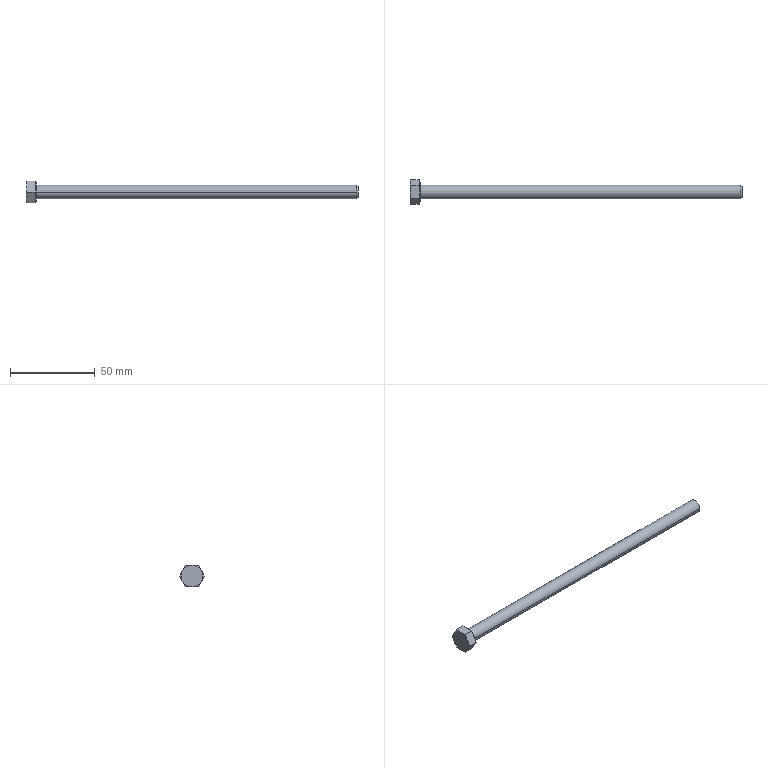Part | SolidWorks | features BaseBody 1 | 1 solid | 28 faces | box 195.95 x 14.699 x 12.73 mm | volume 10367 mm3 | plane 15 | cone 11 | cylinder 2 | commonest cylinder face diameters 8 x2
STEP:
#1=CARTESIAN_POINT('',(195.95,3.324,0.));
#2=VERTEX_POINT('',#1);
#3=CARTESIAN_POINT('',(195.95,-3.323,0.));
#4=VERTEX_POINT('',#3);
#5=CARTESIAN_POINT('',(195.95,0.,0.));
#6=DIRECTION('',(1.,0.,0.));
#7=DIRECTION('',(0.,1.,0.));
#8=AXIS2_PLACEMENT_3D('',#5,#6,#7);
#9=CIRCLE('',#8,3.324);
#10=EDGE_CURVE('',#2,#4,#9,.T.);
#11=ORIENTED_EDGE('',*,*,#10,.F.);
#12=CARTESIAN_POINT('',(195.273,4.,0.));
#13=VERTEX_POINT('',#12);
#14=CARTESIAN_POINT('',(195.95,3.324,0.));
#15=DIRECTION('',(-0.7071,0.7071,0.));
#16=VECTOR('',#15,1000.);
#17=LINE('',#14,#16);
#18=EDGE_CURVE('',#2,#13,#17,.T.);
#19=ORIENTED_EDGE('',*,*,#18,.T.);
#20=CARTESIAN_POINT('',(195.273,-4.,0.));
#21=VERTEX_POINT('',#20);
#22=CARTESIAN_POINT('',(195.273,0.,0.));
#23=DIRECTION('',(-1.,0.,0.));
#24=DIRECTION('',(0.,1.,0.));
#25=AXIS2_PLACEMENT_3D('',#22,#23,#24);
#26=CIRCLE('',#25,4.);
#27=EDGE_CURVE('',#21,#13,#26,.T.);
#28=ORIENTED_EDGE('',*,*,#27,.F.);
#29=CARTESIAN_POINT('',(195.95,-3.323,0.));
#30=DIRECTION('',(-0.7071,-0.7071,0.));
#31=VECTOR('',#30,1000.);
#32=LINE('',#29,#31);
#33=EDGE_CURVE('',#4,#21,#32,.T.);
#34=ORIENTED_EDGE('',*,*,#33,.F.);
#35=EDGE_LOOP('',(#11,#19,#28,#34));
#36=FACE_OUTER_BOUND('',#35,.T.);
#37=CARTESIAN_POINT('',(195.95,0.,0.));
#38=DIRECTION('',(-1.,0.,0.));
#39=DIRECTION('',(0.,-1.,0.));
#40=AXIS2_PLACEMENT_3D('',#37,#38,#39);
#41=CONICAL_SURFACE('',#40,3.324,0.7854);
#42=ADVANCED_FACE('',(#36),#41,.T.);
#43=ORIENTED_EDGE('',*,*,#27,.T.);
#44=CARTESIAN_POINT('',(5.95,4.,0.));
#45=VERTEX_POINT('',#44);
#46=CARTESIAN_POINT('',(195.95,4.,0.));
#47=DIRECTION('',(-1.,0.,0.));
#48=VECTOR('',#47,1000.);
#49=LINE('',#46,#48);
#50=EDGE_CURVE('',#13,#45,#49,.T.);
#51=ORIENTED_EDGE('',*,*,#50,.T.);
#52=CARTESIAN_POINT('',(5.95,-4.,0.));
#53=VERTEX_POINT('',#52);
#54=CARTESIAN_POINT('',(5.95,0.,0.));
#55=DIRECTION('',(1.,0.,0.));
#56=DIRECTION('',(0.,-1.,0.));
#57=AXIS2_PLACEMENT_3D('',#54,#55,#56);
#58=CIRCLE('',#57,4.);
#59=EDGE_CURVE('',#45,#53,#58,.T.);
#60=ORIENTED_EDGE('',*,*,#59,.T.);
#61=CARTESIAN_POINT('',(195.95,-4.,0.));
#62=DIRECTION('',(-1.,0.,0.));
#63=VECTOR('',#62,1000.);
#64=LINE('',#61,#63);
#65=EDGE_CURVE('',#21,#53,#64,.T.);
#66=ORIENTED_EDGE('',*,*,#65,.F.);
#67=EDGE_LOOP('',(#43,#51,#60,#66));
#68=FACE_OUTER_BOUND('',#67,.T.);
#69=CARTESIAN_POINT('',(195.95,0.,0.));
#70=DIRECTION('',(-1.,0.,0.));
#71=DIRECTION('',(0.,-1.,0.));
#72=AXIS2_PLACEMENT_3D('',#69,#70,#71);
#73=CYLINDRICAL_SURFACE('',#72,4.);
#74=ADVANCED_FACE('',(#68),#73,.T.);
#75=CARTESIAN_POINT('',(5.95,-5.815,0.));
#76=VERTEX_POINT('',#75);
#77=CARTESIAN_POINT('',(5.95,5.815,0.));
#78=VERTEX_POINT('',#77);
#79=CARTESIAN_POINT('',(5.95,0.,0.));
#80=DIRECTION('',(-1.,0.,0.));
#81=DIRECTION('',(0.,-1.,0.));
#82=AXIS2_PLACEMENT_3D('',#79,#80,#81);
#83=CIRCLE('',#82,5.815);
#84=EDGE_CURVE('',#76,#78,#83,.T.);
#85=ORIENTED_EDGE('',*,*,#84,.T.);
#86=CARTESIAN_POINT('',(5.45,6.365,0.));
#87=VERTEX_POINT('',#86);
#88=CARTESIAN_POINT('',(5.95,5.815,0.));
#89=DIRECTION('',(-0.6727,0.7399,0.));
#90=VECTOR('',#89,1000.);
#91=LINE('',#88,#90);
#92=EDGE_CURVE('',#78,#87,#91,.T.);
#93=ORIENTED_EDGE('',*,*,#92,.T.);
#94=CARTESIAN_POINT('',(5.45,5.512,3.183));
#95=VERTEX_POINT('',#94);
#96=CARTESIAN_POINT('',(5.45,0.,0.));
#97=DIRECTION('',(-1.,0.,0.));
#98=DIRECTION('',(0.,-1.,0.));
#99=AXIS2_PLACEMENT_3D('',#96,#97,#98);
#100=CIRCLE('',#99,6.365);
#101=EDGE_CURVE('',#95,#87,#100,.T.);
#102=ORIENTED_EDGE('',*,*,#101,.F.);
#103=CARTESIAN_POINT('',(5.45,0.,6.365));
#104=VERTEX_POINT('',#103);
#105=CARTESIAN_POINT('',(5.45,0.,0.));
#106=DIRECTION('',(-1.,0.,0.));
#107=DIRECTION('',(0.,-1.,0.));
#108=AXIS2_PLACEMENT_3D('',#105,#106,#107);
#109=CIRCLE('',#108,6.365);
#110=EDGE_CURVE('',#104,#95,#109,.T.);
#111=ORIENTED_EDGE('',*,*,#110,.F.);
#112=CARTESIAN_POINT('',(5.45,-5.512,3.183));
#113=VERTEX_POINT('',#112);
#114=CARTESIAN_POINT('',(5.45,0.,0.));
#115=DIRECTION('',(-1.,0.,0.));
#116=DIRECTION('',(0.,-1.,0.));
#117=AXIS2_PLACEMENT_3D('',#114,#115,#116);
#118=CIRCLE('',#117,6.365);
#119=EDGE_CURVE('',#113,#104,#118,.T.);
#120=ORIENTED_EDGE('',*,*,#119,.F.);
#121=CARTESIAN_POINT('',(5.45,-6.365,0.));
#122=VERTEX_POINT('',#121);
#123=CARTESIAN_POINT('',(5.45,0.,0.));
#124=DIRECTION('',(-1.,0.,0.));
#125=DIRECTION('',(0.,-1.,0.));
#126=AXIS2_PLACEMENT_3D('',#123,#124,#125);
#127=CIRCLE('',#126,6.365);
#128=EDGE_CURVE('',#122,#113,#127,.T.);
#129=ORIENTED_EDGE('',*,*,#128,.F.);
#130=CARTESIAN_POINT('',(5.95,-5.815,0.));
#131=DIRECTION('',(-0.6727,-0.7399,0.));
#132=VECTOR('',#131,1000.);
#133=LINE('',#130,#132);
#134=EDGE_CURVE('',#76,#122,#133,.T.);
#135=ORIENTED_EDGE('',*,*,#134,.F.);
#136=EDGE_LOOP('',(#85,#93,#102,#111,#120,#129,#135));
#137=FACE_OUTER_BOUND('',#136,.T.);
#138=CARTESIAN_POINT('',(5.95,0.,0.));
#139=DIRECTION('',(-1.,0.,0.));
#140=DIRECTION('',(0.,-1.,0.));
#141=AXIS2_PLACEMENT_3D('',#138,#139,#140);
#142=CONICAL_SURFACE('',#141,5.815,0.833);
#143=ADVANCED_FACE('',(#137),#142,.T.);
#144=CARTESIAN_POINT('',(0.,6.365,0.));
#145=VERTEX_POINT('',#144);
#146=CARTESIAN_POINT('',(0.,5.512,-3.183));
#147=VERTEX_POINT('',#146);
#148=CARTESIAN_POINT('',(0.,0.,0.));
#149=DIRECTION('',(-1.,0.,0.));
#150=DIRECTION('',(0.,0.,1.));
#151=AXIS2_PLACEMENT_3D('',#148,#149,#150);
#152=CIRCLE('',#151,6.365);
#153=EDGE_CURVE('',#145,#147,#152,.T.);
#154=ORIENTED_EDGE('',*,*,#153,.F.);
#155=CARTESIAN_POINT('',(0.3584,7.35,0.));
#156=VERTEX_POINT('',#155);
#157=CARTESIAN_POINT('',(0.,6.365,0.));
#158=DIRECTION('',(0.342,0.9397,0.));
#159=VECTOR('',#158,1000.);
#160=LINE('',#157,#159);
#161=EDGE_CURVE('',#145,#156,#160,.T.);
#162=ORIENTED_EDGE('',*,*,#161,.T.);
#163=CARTESIAN_POINT('',(0.3584,7.35,0.));
#164=CARTESIAN_POINT('',(0.3008,7.191,-0.2742));
#165=CARTESIAN_POINT('',(0.25,7.037,-0.5421));
#166=CARTESIAN_POINT('',(0.184,6.808,-0.9385));
#167=CARTESIAN_POINT('',(0.1638,6.732,-1.07));
#168=CARTESIAN_POINT('',(0.1359,6.619,-1.266));
#169=CARTESIAN_POINT('',(0.127,6.581,-1.331));
#170=CARTESIAN_POINT('',(0.1102,6.506,-1.461));
#171=CARTESIAN_POINT('',(0.1024,6.47,-1.524));
#172=CARTESIAN_POINT('',(0.07901,6.354,-1.725));
#173=CARTESIAN_POINT('',(0.06534,6.277,-1.858));
#174=CARTESIAN_POINT('',(0.04182,6.124,-2.123));
#175=CARTESIAN_POINT('',(0.03203,6.049,-2.254));
#176=CARTESIAN_POINT('',(0.008007,5.818,-2.654));
#177=CARTESIAN_POINT('',(0.,5.666,-2.917));
#178=CARTESIAN_POINT('',(0.,5.512,-3.183));
#179=B_SPLINE_CURVE_WITH_KNOTS('',3,(#163,#164,#165,#166,#167,#168,#169,#170,#171,#172,#173,#174,#175,#176,#177,#178),.UNSPECIFIED.,.F.,.F.,(4,2,2,2,2,2,2,4),(0.,0.25,0.375,0.4375,0.5,0.625,0.75,1.),.UNSPECIFIED.);
#180=EDGE_CURVE('',#156,#147,#179,.T.);
#181=ORIENTED_EDGE('',*,*,#180,.T.);
#182=EDGE_LOOP('',(#154,#162,#181));
#183=FACE_OUTER_BOUND('',#182,.T.);
#184=CARTESIAN_POINT('',(0.,0.,0.));
#185=DIRECTION('',(1.,0.,0.));
#186=DIRECTION('',(0.,1.,0.));
#187=AXIS2_PLACEMENT_3D('',#184,#185,#186);
#188=CONICAL_SURFACE('',#187,6.365,1.222);
#189=ADVANCED_FACE('',(#183),#188,.T.);
#190=ORIENTED_EDGE('',*,*,#84,.F.);
#191=CARTESIAN_POINT('',(5.95,0.,0.));
#192=DIRECTION('',(-1.,0.,0.));
#193=DIRECTION('',(0.,-1.,0.));
#194=AXIS2_PLACEMENT_3D('',#191,#192,#193);
#195=CIRCLE('',#194,5.815);
#196=EDGE_CURVE('',#78,#76,#195,.T.);
#197=ORIENTED_EDGE('',*,*,#196,.F.);
#198=EDGE_LOOP('',(#190,#197));
#199=FACE_OUTER_BOUND('',#198,.T.);
#200=CARTESIAN_POINT('',(5.95,0.,0.));
#201=DIRECTION('',(1.,0.,0.));
#202=DIRECTION('',(0.,-1.,0.));
#203=AXIS2_PLACEMENT_3D('',#200,#201,#202);
#204=CIRCLE('',#203,4.);
#205=EDGE_CURVE('',#53,#45,#204,.T.);
#206=ORIENTED_EDGE('',*,*,#205,.F.);
#207=ORIENTED_EDGE('',*,*,#59,.F.);
#208=EDGE_LOOP('',(#206,#207));
#209=FACE_BOUND('',#208,.T.);
#210=CARTESIAN_POINT('',(5.95,0.,0.));
#211=DIRECTION('',(-1.,0.,0.));
#212=DIRECTION('',(0.,1.,0.));
#213=AXIS2_PLACEMENT_3D('',#210,#211,#212);
#214=PLANE('',#213);
#215=ADVANCED_FACE('',(#199,#209),#214,.F.);
#216=CARTESIAN_POINT('',(5.45,-3.675,6.365));
#217=VERTEX_POINT('',#216);
#218=CARTESIAN_POINT('',(5.45,-3.675,6.365));
#219=DIRECTION('',(0.,-0.5,-0.866));
#220=VECTOR('',#219,1000.);
#221=LINE('',#218,#220);
#222=EDGE_CURVE('',#217,#113,#221,.T.);
#223=ORIENTED_EDGE('',*,*,#222,.T.);
#224=ORIENTED_EDGE('',*,*,#119,.T.);
#225=CARTESIAN_POINT('',(5.45,3.675,6.365));
#226=DIRECTION('',(0.,-1.,0.));
#227=VECTOR('',#226,1000.);
#228=LINE('',#225,#227);
#229=EDGE_CURVE('',#104,#217,#228,.T.);
#230=ORIENTED_EDGE('',*,*,#229,.T.);
#231=EDGE_LOOP('',(#223,#224,#230));
#232=FACE_OUTER_BOUND('',#231,.T.);
#233=CARTESIAN_POINT('',(5.45,0.,12.73));
#234=DIRECTION('',(-1.,0.,0.));
#235=DIRECTION('',(0.,0.,1.));
#236=AXIS2_PLACEMENT_3D('',#233,#234,#235);
#237=PLANE('',#236);
#238=ADVANCED_FACE('',(#232),#237,.F.);
#239=CARTESIAN_POINT('',(5.45,3.675,6.365));
#240=VERTEX_POINT('',#239);
#241=CARTESIAN_POINT('',(5.45,3.675,6.365));
#242=DIRECTION('',(0.,-1.,0.));
#243=VECTOR('',#242,1000.);
#244=LINE('',#241,#243);
#245=EDGE_CURVE('',#240,#104,#244,.T.);
#246=ORIENTED_EDGE('',*,*,#245,.T.);
#247=ORIENTED_EDGE('',*,*,#110,.T.);
#248=CARTESIAN_POINT('',(5.45,7.35,0.));
#249=DIRECTION('',(0.,-0.5,0.866));
#250=VECTOR('',#249,1000.);
#251=LINE('',#248,#250);
#252=EDGE_CURVE('',#95,#240,#251,.T.);
#253=ORIENTED_EDGE('',*,*,#252,.T.);
#254=EDGE_LOOP('',(#246,#247,#253));
#255=FACE_OUTER_BOUND('',#254,.T.);
#256=CARTESIAN_POINT('',(5.45,0.,12.73));
#257=DIRECTION('',(-1.,0.,0.));
#258=DIRECTION('',(0.,0.,1.));
#259=AXIS2_PLACEMENT_3D('',#256,#257,#258);
#260=PLANE('',#259);
#261=ADVANCED_FACE('',(#255),#260,.F.);
#262=CARTESIAN_POINT('',(5.45,7.35,0.));
#263=VERTEX_POINT('',#262);
#264=CARTESIAN_POINT('',(5.45,7.35,0.));
#265=DIRECTION('',(0.,-0.5,0.866));
#266=VECTOR('',#265,1000.);
#267=LINE('',#264,#266);
#268=EDGE_CURVE('',#263,#95,#267,.T.);
#269=ORIENTED_EDGE('',*,*,#268,.T.);
#270=ORIENTED_EDGE('',*,*,#101,.T.);
#271=CARTESIAN_POINT('',(5.45,5.512,-3.183));
#272=VERTEX_POINT('',#271);
#273=CARTESIAN_POINT('',(5.45,0.,0.));
#274=DIRECTION('',(-1.,0.,0.));
#275=DIRECTION('',(0.,-1.,0.));
#276=AXIS2_PLACEMENT_3D('',#273,#274,#275);
#277=CIRCLE('',#276,6.365);
#278=EDGE_CURVE('',#87,#272,#277,.T.);
#279=ORIENTED_EDGE('',*,*,#278,.T.);
#280=CARTESIAN_POINT('',(5.45,3.675,-6.365));
#281=DIRECTION('',(0.,0.5,0.866));
#282=VECTOR('',#281,1000.);
#283=LINE('',#280,#282);
#284=EDGE_CURVE('',#272,#263,#283,.T.);
#285=ORIENTED_EDGE('',*,*,#284,.T.);
#286=EDGE_LOOP('',(#269,#270,#279,#285));
#287=FACE_OUTER_BOUND('',#286,.T.);
#288=CARTESIAN_POINT('',(5.45,0.,12.73));
#289=DIRECTION('',(-1.,0.,0.));
#290=DIRECTION('',(0.,0.,1.));
#291=AXIS2_PLACEMENT_3D('',#288,#289,#290);
#292=PLANE('',#291);
#293=ADVANCED_FACE('',(#287),#292,.F.);
#294=CARTESIAN_POINT('',(5.45,3.675,-6.365));
#295=VERTEX_POINT('',#294);
#296=CARTESIAN_POINT('',(5.45,3.675,-6.365));
#297=DIRECTION('',(0.,0.5,0.866));
#298=VECTOR('',#297,1000.);
#299=LINE('',#296,#298);
#300=EDGE_CURVE('',#295,#272,#299,.T.);
#301=ORIENTED_EDGE('',*,*,#300,.T.);
#302=CARTESIAN_POINT('',(5.45,0.,-6.365));
#303=VERTEX_POINT('',#302);
#304=CARTESIAN_POINT('',(5.45,0.,0.));
#305=DIRECTION('',(-1.,0.,0.));
#306=DIRECTION('',(0.,-1.,0.));
#307=AXIS2_PLACEMENT_3D('',#304,#305,#306);
#308=CIRCLE('',#307,6.365);
#309=EDGE_CURVE('',#272,#303,#308,.T.);
#310=ORIENTED_EDGE('',*,*,#309,.T.);
#311=CARTESIAN_POINT('',(5.45,-3.675,-6.365));
#312=DIRECTION('',(0.,1.,0.));
#313=VECTOR('',#312,1000.);
#314=LINE('',#311,#313);
#315=EDGE_CURVE('',#303,#295,#314,.T.);
#316=ORIENTED_EDGE('',*,*,#315,.T.);
#317=EDGE_LOOP('',(#301,#310,#316));
#318=FACE_OUTER_BOUND('',#317,.T.);
#319=CARTESIAN_POINT('',(5.45,0.,12.73));
#320=DIRECTION('',(-1.,0.,0.));
#321=DIRECTION('',(0.,0.,1.));
#322=AXIS2_PLACEMENT_3D('',#319,#320,#321);
#323=PLANE('',#322);
#324=ADVANCED_FACE('',(#318),#323,.F.);
#325=CARTESIAN_POINT('',(5.45,-3.675,-6.365));
#326=VERTEX_POINT('',#325);
#327=CARTESIAN_POINT('',(5.45,-3.675,-6.365));
#328=DIRECTION('',(0.,1.,0.));
#329=VECTOR('',#328,1000.);
#330=LINE('',#327,#329);
#331=EDGE_CURVE('',#326,#303,#330,.T.);
#332=ORIENTED_EDGE('',*,*,#331,.T.);
#333=CARTESIAN_POINT('',(5.45,-5.512,-3.183));
#334=VERTEX_POINT('',#333);
#335=CARTESIAN_POINT('',(5.45,0.,0.));
#336=DIRECTION('',(-1.,0.,0.));
#337=DIRECTION('',(0.,-1.,0.));
#338=AXIS2_PLACEMENT_3D('',#335,#336,#337);
#339=CIRCLE('',#338,6.365);
#340=EDGE_CURVE('',#303,#334,#339,.T.);
#341=ORIENTED_EDGE('',*,*,#340,.T.);
#342=CARTESIAN_POINT('',(5.45,-7.35,0.));
#343=DIRECTION('',(0.,0.5,-0.866));
#344=VECTOR('',#343,1000.);
#345=LINE('',#342,#344);
#346=EDGE_CURVE('',#334,#326,#345,.T.);
#347=ORIENTED_EDGE('',*,*,#346,.T.);
#348=EDGE_LOOP('',(#332,#341,#347));
#349=FACE_OUTER_BOUND('',#348,.T.);
#350=CARTESIAN_POINT('',(5.45,0.,12.73));
#351=DIRECTION('',(-1.,0.,0.));
#352=DIRECTION('',(0.,0.,1.));
#353=AXIS2_PLACEMENT_3D('',#350,#351,#352);
#354=PLANE('',#353);
#355=ADVANCED_FACE('',(#349),#354,.F.);
#356=CARTESIAN_POINT('',(0.3584,-7.35,0.));
#357=VERTEX_POINT('',#356);
#358=CARTESIAN_POINT('',(0.,-5.512,3.183));
#359=VERTEX_POINT('',#358);
#360=CARTESIAN_POINT('',(0.3584,-7.35,0.));
#361=CARTESIAN_POINT('',(0.3008,-7.191,0.2742));
#362=CARTESIAN_POINT('',(0.25,-7.037,0.5421));
#363=CARTESIAN_POINT('',(0.184,-6.808,0.9385));
#364=CARTESIAN_POINT('',(0.1638,-6.732,1.07));
#365=CARTESIAN_POINT('',(0.1359,-6.619,1.266));
#366=CARTESIAN_POINT('',(0.127,-6.581,1.331));
#367=CARTESIAN_POINT('',(0.1102,-6.506,1.461));
#368=CARTESIAN_POINT('',(0.1024,-6.47,1.524));
#369=CARTESIAN_POINT('',(0.07901,-6.354,1.725));
#370=CARTESIAN_POINT('',(0.06534,-6.277,1.858));
#371=CARTESIAN_POINT('',(0.04182,-6.124,2.123));
#372=CARTESIAN_POINT('',(0.03203,-6.049,2.254));
#373=CARTESIAN_POINT('',(0.008007,-5.818,2.654));
#374=CARTESIAN_POINT('',(0.,-5.666,2.917));
#375=CARTESIAN_POINT('',(0.,-5.512,3.183));
#376=B_SPLINE_CURVE_WITH_KNOTS('',3,(#360,#361,#362,#363,#364,#365,#366,#367,#368,#369,#370,#371,#372,#373,#374,#375),.UNSPECIFIED.,.F.,.F.,(4,2,2,2,2,2,2,4),(0.,0.25,0.375,0.4375,0.5,0.625,0.75,1.),.UNSPECIFIED.);
#377=EDGE_CURVE('',#357,#359,#376,.T.);
#378=ORIENTED_EDGE('',*,*,#377,.F.);
#379=CARTESIAN_POINT('',(5.45,-7.35,0.));
#380=VERTEX_POINT('',#379);
#381=CARTESIAN_POINT('',(5.45,-7.35,0.));
#382=DIRECTION('',(-1.,0.,0.));
#383=VECTOR('',#382,1000.);
#384=LINE('',#381,#383);
#385=EDGE_CURVE('',#380,#357,#384,.T.);
#386=ORIENTED_EDGE('',*,*,#385,.F.);
#387=CARTESIAN_POINT('',(5.45,-3.675,6.365));
#388=DIRECTION('',(0.,-0.5,-0.866));
#389=VECTOR('',#388,1000.);
#390=LINE('',#387,#389);
#391=EDGE_CURVE('',#113,#380,#390,.T.);
#392=ORIENTED_EDGE('',*,*,#391,.F.);
#393=ORIENTED_EDGE('',*,*,#222,.F.);
#394=CARTESIAN_POINT('',(0.3584,-3.675,6.365));
#395=VERTEX_POINT('',#394);
#396=CARTESIAN_POINT('',(5.45,-3.675,6.365));
#397=DIRECTION('',(-1.,0.,0.));
#398=VECTOR('',#397,1000.);
#399=LINE('',#396,#398);
#400=EDGE_CURVE('',#217,#395,#399,.T.);
#401=ORIENTED_EDGE('',*,*,#400,.T.);
#402=CARTESIAN_POINT('',(0.,-5.512,3.183));
#403=CARTESIAN_POINT('',(0.,-5.436,3.315));
#404=CARTESIAN_POINT('',(0.002002,-5.359,3.447));
#405=CARTESIAN_POINT('',(0.01001,-5.206,3.712));
#406=CARTESIAN_POINT('',(0.01608,-5.129,3.846));
#407=CARTESIAN_POINT('',(0.03196,-4.977,4.11));
#408=CARTESIAN_POINT('',(0.04181,-4.9,4.242));
#409=CARTESIAN_POINT('',(0.05946,-4.786,4.441));
#410=CARTESIAN_POINT('',(0.06582,-4.747,4.507));
#411=CARTESIAN_POINT('',(0.07949,-4.671,4.64));
#412=CARTESIAN_POINT('',(0.08702,-4.631,4.709));
#413=CARTESIAN_POINT('',(0.1552,-4.293,5.294));
#414=CARTESIAN_POINT('',(0.2431,-3.991,5.817));
#415=CARTESIAN_POINT('',(0.3584,-3.675,6.365));
#416=B_SPLINE_CURVE_WITH_KNOTS('',3,(#402,#403,#404,#405,#406,#407,#408,#409,#410,#411,#412,#413,#414,#415),.UNSPECIFIED.,.F.,.F.,(4,2,2,2,2,2,4),(0.,0.125,0.25,0.375,0.4375,0.5,1.),.UNSPECIFIED.);
#417=EDGE_CURVE('',#359,#395,#416,.T.);
#418=ORIENTED_EDGE('',*,*,#417,.F.);
#419=EDGE_LOOP('',(#378,#386,#392,#393,#401,#418));
#420=FACE_OUTER_BOUND('',#419,.T.);
#421=CARTESIAN_POINT('',(5.45,-3.675,6.365));
#422=DIRECTION('',(0.,0.866,-0.5));
#423=DIRECTION('',(-1.,0.,0.));
#424=AXIS2_PLACEMENT_3D('',#421,#422,#423);
#425=PLANE('',#424);
#426=ADVANCED_FACE('',(#420),#425,.F.);
#427=CARTESIAN_POINT('',(0.3584,-3.675,-6.365));
#428=VERTEX_POINT('',#427);
#429=CARTESIAN_POINT('',(0.,-5.512,-3.183));
#430=VERTEX_POINT('',#429);
#431=CARTESIAN_POINT('',(0.3584,-3.675,-6.365));
#432=CARTESIAN_POINT('',(0.3008,-3.833,-6.091));
#433=CARTESIAN_POINT('',(0.25,-3.988,-5.823));
#434=CARTESIAN_POINT('',(0.184,-4.217,-5.426));
#435=CARTESIAN_POINT('',(0.1638,-4.292,-5.295));
#436=CARTESIAN_POINT('',(0.1359,-4.406,-5.099));
#437=CARTESIAN_POINT('',(0.127,-4.443,-5.034));
#438=CARTESIAN_POINT('',(0.1102,-4.518,-4.904));
#439=CARTESIAN_POINT('',(0.1024,-4.555,-4.841));
#440=CARTESIAN_POINT('',(0.07901,-4.671,-4.64));
#441=CARTESIAN_POINT('',(0.06534,-4.747,-4.507));
#442=CARTESIAN_POINT('',(0.04182,-4.9,-4.242));
#443=CARTESIAN_POINT('',(0.03203,-4.976,-4.111));
#444=CARTESIAN_POINT('',(0.008007,-5.207,-3.711));
#445=CARTESIAN_POINT('',(0.,-5.359,-3.448));
#446=CARTESIAN_POINT('',(0.,-5.512,-3.183));
#447=B_SPLINE_CURVE_WITH_KNOTS('',3,(#431,#432,#433,#434,#435,#436,#437,#438,#439,#440,#441,#442,#443,#444,#445,#446),.UNSPECIFIED.,.F.,.F.,(4,2,2,2,2,2,2,4),(0.,0.25,0.375,0.4375,0.5,0.625,0.75,1.),.UNSPECIFIED.);
#448=EDGE_CURVE('',#428,#430,#447,.T.);
#449=ORIENTED_EDGE('',*,*,#448,.F.);
#450=CARTESIAN_POINT('',(5.45,-3.675,-6.365));
#451=DIRECTION('',(-1.,0.,0.));
#452=VECTOR('',#451,1000.);
#453=LINE('',#450,#452);
#454=EDGE_CURVE('',#326,#428,#453,.T.);
#455=ORIENTED_EDGE('',*,*,#454,.F.);
#456=ORIENTED_EDGE('',*,*,#346,.F.);
#457=CARTESIAN_POINT('',(5.45,-7.35,0.));
#458=DIRECTION('',(0.,0.5,-0.866));
#459=VECTOR('',#458,1000.);
#460=LINE('',#457,#459);
#461=EDGE_CURVE('',#380,#334,#460,.T.);
#462=ORIENTED_EDGE('',*,*,#461,.F.);
#463=ORIENTED_EDGE('',*,*,#385,.T.);
#464=CARTESIAN_POINT('',(0.,-5.512,-3.183));
#465=CARTESIAN_POINT('',(0.,-5.589,-3.05));
#466=CARTESIAN_POINT('',(0.002002,-5.665,-2.918));
#467=CARTESIAN_POINT('',(0.01001,-5.818,-2.653));
#468=CARTESIAN_POINT('',(0.01608,-5.895,-2.519));
#469=CARTESIAN_POINT('',(0.03196,-6.048,-2.255));
#470=CARTESIAN_POINT('',(0.04181,-6.124,-2.123));
#471=CARTESIAN_POINT('',(0.05946,-6.239,-1.924));
#472=CARTESIAN_POINT('',(0.06582,-6.277,-1.858));
#473=CARTESIAN_POINT('',(0.07949,-6.354,-1.725));
#474=CARTESIAN_POINT('',(0.08702,-6.393,-1.656));
#475=CARTESIAN_POINT('',(0.1552,-6.731,-1.071));
#476=CARTESIAN_POINT('',(0.2431,-7.033,-0.5484));
#477=CARTESIAN_POINT('',(0.3584,-7.35,0.));
#478=B_SPLINE_CURVE_WITH_KNOTS('',3,(#464,#465,#466,#467,#468,#469,#470,#471,#472,#473,#474,#475,#476,#477),.UNSPECIFIED.,.F.,.F.,(4,2,2,2,2,2,4),(0.,0.125,0.25,0.375,0.4375,0.5,1.),.UNSPECIFIED.);
#479=EDGE_CURVE('',#430,#357,#478,.T.);
#480=ORIENTED_EDGE('',*,*,#479,.F.);
#481=EDGE_LOOP('',(#449,#455,#456,#462,#463,#480));
#482=FACE_OUTER_BOUND('',#481,.T.);
#483=CARTESIAN_POINT('',(5.45,-7.35,0.));
#484=DIRECTION('',(0.,0.866,0.5));
#485=DIRECTION('',(1.,0.,0.));
#486=AXIS2_PLACEMENT_3D('',#483,#484,#485);
#487=PLANE('',#486);
#488=ADVANCED_FACE('',(#482),#487,.F.);
#489=CARTESIAN_POINT('',(0.3584,3.675,-6.365));
#490=VERTEX_POINT('',#489);
#491=CARTESIAN_POINT('',(0.,0.,-6.365));
#492=VERTEX_POINT('',#491);
#493=CARTESIAN_POINT('',(0.3584,3.675,-6.365));
#494=CARTESIAN_POINT('',(0.3008,3.359,-6.365));
#495=CARTESIAN_POINT('',(0.2501,3.049,-6.365));
#496=CARTESIAN_POINT('',(0.1842,2.592,-6.365));
#497=CARTESIAN_POINT('',(0.1639,2.441,-6.365));
#498=CARTESIAN_POINT('',(0.1361,2.215,-6.365));
#499=CARTESIAN_POINT('',(0.1272,2.139,-6.365));
#500=CARTESIAN_POINT('',(0.1104,1.989,-6.365));
#501=CARTESIAN_POINT('',(0.1026,1.916,-6.365));
#502=CARTESIAN_POINT('',(0.07918,1.685,-6.365));
#503=CARTESIAN_POINT('',(0.06548,1.531,-6.365));
#504=CARTESIAN_POINT('',(0.04192,1.225,-6.365));
#505=CARTESIAN_POINT('',(0.03212,1.074,-6.365));
#506=CARTESIAN_POINT('',(0.008031,0.6117,-6.365));
#507=CARTESIAN_POINT('',(0.,0.3071,-6.365));
#508=CARTESIAN_POINT('',(0.,0.,-6.365));
#509=B_SPLINE_CURVE_WITH_KNOTS('',3,(#493,#494,#495,#496,#497,#498,#499,#500,#501,#502,#503,#504,#505,#506,#507,#508),.UNSPECIFIED.,.F.,.F.,(4,2,2,2,2,2,2,4),(0.,0.25,0.375,0.4375,0.5,0.625,0.75,1.),.UNSPECIFIED.);
#510=EDGE_CURVE('',#490,#492,#509,.T.);
#511=ORIENTED_EDGE('',*,*,#510,.F.);
#512=CARTESIAN_POINT('',(5.45,3.675,-6.365));
#513=DIRECTION('',(-1.,0.,0.));
#514=VECTOR('',#513,1000.);
#515=LINE('',#512,#514);
#516=EDGE_CURVE('',#295,#490,#515,.T.);
#517=ORIENTED_EDGE('',*,*,#516,.F.);
#518=ORIENTED_EDGE('',*,*,#315,.F.);
#519=ORIENTED_EDGE('',*,*,#331,.F.);
#520=ORIENTED_EDGE('',*,*,#454,.T.);
#521=CARTESIAN_POINT('',(0.,0.,-6.365));
#522=CARTESIAN_POINT('',(0.,-0.3065,-6.365));
#523=CARTESIAN_POINT('',(0.008117,-0.6128,-6.365));
#524=CARTESIAN_POINT('',(0.03195,-1.071,-6.365));
#525=CARTESIAN_POINT('',(0.04181,-1.224,-6.365));
#526=CARTESIAN_POINT('',(0.05947,-1.453,-6.365));
#527=CARTESIAN_POINT('',(0.06584,-1.53,-6.365));
#528=CARTESIAN_POINT('',(0.07952,-1.684,-6.365));
#529=CARTESIAN_POINT('',(0.08707,-1.763,-6.365));
#530=CARTESIAN_POINT('',(0.1553,-2.438,-6.365));
#531=CARTESIAN_POINT('',(0.2432,-3.042,-6.365));
#532=CARTESIAN_POINT('',(0.3584,-3.675,-6.365));
#533=B_SPLINE_CURVE_WITH_KNOTS('',3,(#521,#522,#523,#524,#525,#526,#527,#528,#529,#530,#531,#532),.UNSPECIFIED.,.F.,.F.,(4,2,2,2,2,4),(0.,0.25,0.375,0.4375,0.5,1.),.UNSPECIFIED.);
#534=EDGE_CURVE('',#492,#428,#533,.T.);
#535=ORIENTED_EDGE('',*,*,#534,.F.);
#536=EDGE_LOOP('',(#511,#517,#518,#519,#520,#535));
#537=FACE_OUTER_BOUND('',#536,.T.);
#538=CARTESIAN_POINT('',(5.45,-3.675,-6.365));
#539=DIRECTION('',(0.,0.,1.));
#540=DIRECTION('',(0.,-1.,0.));
#541=AXIS2_PLACEMENT_3D('',#538,#539,#540);
#542=PLANE('',#541);
#543=ADVANCED_FACE('',(#537),#542,.F.);
#544=ORIENTED_EDGE('',*,*,#180,.F.);
#545=CARTESIAN_POINT('',(5.45,7.35,0.));
#546=DIRECTION('',(-1.,0.,0.));
#547=VECTOR('',#546,1000.);
#548=LINE('',#545,#547);
#549=EDGE_CURVE('',#263,#156,#548,.T.);
#550=ORIENTED_EDGE('',*,*,#549,.F.);
#551=ORIENTED_EDGE('',*,*,#284,.F.);
#552=ORIENTED_EDGE('',*,*,#300,.F.);
#553=ORIENTED_EDGE('',*,*,#516,.T.);
#554=CARTESIAN_POINT('',(0.,5.512,-3.183));
#555=CARTESIAN_POINT('',(0.,5.436,-3.315));
#556=CARTESIAN_POINT('',(0.002002,5.359,-3.447));
#557=CARTESIAN_POINT('',(0.01001,5.206,-3.712));
#558=CARTESIAN_POINT('',(0.01608,5.129,-3.846));
#559=CARTESIAN_POINT('',(0.03196,4.977,-4.11));
#560=CARTESIAN_POINT('',(0.04181,4.9,-4.242));
#561=CARTESIAN_POINT('',(0.05946,4.786,-4.441));
#562=CARTESIAN_POINT('',(0.06582,4.747,-4.507));
#563=CARTESIAN_POINT('',(0.07949,4.671,-4.64));
#564=CARTESIAN_POINT('',(0.08702,4.631,-4.709));
#565=CARTESIAN_POINT('',(0.1552,4.293,-5.294));
#566=CARTESIAN_POINT('',(0.2431,3.991,-5.817));
#567=CARTESIAN_POINT('',(0.3584,3.675,-6.365));
#568=B_SPLINE_CURVE_WITH_KNOTS('',3,(#554,#555,#556,#557,#558,#559,#560,#561,#562,#563,#564,#565,#566,#567),.UNSPECIFIED.,.F.,.F.,(4,2,2,2,2,2,4),(0.,0.125,0.25,0.375,0.4375,0.5,1.),.UNSPECIFIED.);
#569=EDGE_CURVE('',#147,#490,#568,.T.);
#570=ORIENTED_EDGE('',*,*,#569,.F.);
#571=EDGE_LOOP('',(#544,#550,#551,#552,#553,#570));
#572=FACE_OUTER_BOUND('',#571,.T.);
#573=CARTESIAN_POINT('',(5.45,3.675,-6.365));
#574=DIRECTION('',(0.,-0.866,0.5));
#575=DIRECTION('',(-1.,0.,0.));
#576=AXIS2_PLACEMENT_3D('',#573,#574,#575);
#577=PLANE('',#576);
#578=ADVANCED_FACE('',(#572),#577,.F.);
#579=CARTESIAN_POINT('',(0.3584,3.675,6.365));
#580=VERTEX_POINT('',#579);
#581=CARTESIAN_POINT('',(0.,5.512,3.183));
#582=VERTEX_POINT('',#581);
#583=CARTESIAN_POINT('',(0.3584,3.675,6.365));
#584=CARTESIAN_POINT('',(0.3008,3.833,6.091));
#585=CARTESIAN_POINT('',(0.25,3.988,5.823));
#586=CARTESIAN_POINT('',(0.184,4.217,5.426));
#587=CARTESIAN_POINT('',(0.1638,4.292,5.295));
#588=CARTESIAN_POINT('',(0.1359,4.406,5.099));
#589=CARTESIAN_POINT('',(0.127,4.443,5.034));
#590=CARTESIAN_POINT('',(0.1102,4.518,4.904));
#591=CARTESIAN_POINT('',(0.1024,4.555,4.841));
#592=CARTESIAN_POINT('',(0.07901,4.671,4.64));
#593=CARTESIAN_POINT('',(0.06534,4.747,4.507));
#594=CARTESIAN_POINT('',(0.04182,4.9,4.242));
#595=CARTESIAN_POINT('',(0.03203,4.976,4.111));
#596=CARTESIAN_POINT('',(0.008007,5.207,3.711));
#597=CARTESIAN_POINT('',(0.,5.359,3.448));
#598=CARTESIAN_POINT('',(0.,5.512,3.183));
#599=B_SPLINE_CURVE_WITH_KNOTS('',3,(#583,#584,#585,#586,#587,#588,#589,#590,#591,#592,#593,#594,#595,#596,#597,#598),.UNSPECIFIED.,.F.,.F.,(4,2,2,2,2,2,2,4),(0.,0.25,0.375,0.4375,0.5,0.625,0.75,1.),.UNSPECIFIED.);
#600=EDGE_CURVE('',#580,#582,#599,.T.);
#601=ORIENTED_EDGE('',*,*,#600,.F.);
#602=CARTESIAN_POINT('',(5.45,3.675,6.365));
#603=DIRECTION('',(-1.,0.,0.));
#604=VECTOR('',#603,1000.);
#605=LINE('',#602,#604);
#606=EDGE_CURVE('',#240,#580,#605,.T.);
#607=ORIENTED_EDGE('',*,*,#606,.F.);
#608=ORIENTED_EDGE('',*,*,#252,.F.);
#609=ORIENTED_EDGE('',*,*,#268,.F.);
#610=ORIENTED_EDGE('',*,*,#549,.T.);
#611=CARTESIAN_POINT('',(0.,5.512,3.183));
#612=CARTESIAN_POINT('',(0.,5.589,3.05));
#613=CARTESIAN_POINT('',(0.002002,5.665,2.918));
#614=CARTESIAN_POINT('',(0.01001,5.818,2.653));
#615=CARTESIAN_POINT('',(0.01608,5.895,2.519));
#616=CARTESIAN_POINT('',(0.03196,6.048,2.255));
#617=CARTESIAN_POINT('',(0.04181,6.124,2.123));
#618=CARTESIAN_POINT('',(0.05946,6.239,1.924));
#619=CARTESIAN_POINT('',(0.06582,6.277,1.858));
#620=CARTESIAN_POINT('',(0.07949,6.354,1.725));
#621=CARTESIAN_POINT('',(0.08702,6.393,1.656));
#622=CARTESIAN_POINT('',(0.1552,6.731,1.071));
#623=CARTESIAN_POINT('',(0.2431,7.033,0.5484));
#624=CARTESIAN_POINT('',(0.3584,7.35,0.));
#625=B_SPLINE_CURVE_WITH_KNOTS('',3,(#611,#612,#613,#614,#615,#616,#617,#618,#619,#620,#621,#622,#623,#624),.UNSPECIFIED.,.F.,.F.,(4,2,2,2,2,2,4),(0.,0.125,0.25,0.375,0.4375,0.5,1.),.UNSPECIFIED.);
#626=EDGE_CURVE('',#582,#156,#625,.T.);
#627=ORIENTED_EDGE('',*,*,#626,.F.);
#628=EDGE_LOOP('',(#601,#607,#608,#609,#610,#627));
#629=FACE_OUTER_BOUND('',#628,.T.);
#630=CARTESIAN_POINT('',(5.45,7.35,0.));
#631=DIRECTION('',(0.,-0.866,-0.5));
#632=DIRECTION('',(0.,0.5,-0.866));
#633=AXIS2_PLACEMENT_3D('',#630,#631,#632);
#634=PLANE('',#633);
#635=ADVANCED_FACE('',(#629),#634,.F.);
#636=CARTESIAN_POINT('',(0.,0.,6.365));
#637=VERTEX_POINT('',#636);
#638=CARTESIAN_POINT('',(0.3584,-3.675,6.365));
#639=CARTESIAN_POINT('',(0.3008,-3.358,6.365));
#640=CARTESIAN_POINT('',(0.25,-3.049,6.365));
#641=CARTESIAN_POINT('',(0.1841,-2.591,6.365));
#642=CARTESIAN_POINT('',(0.1638,-2.44,6.365));
#643=CARTESIAN_POINT('',(0.136,-2.214,6.365));
#644=CARTESIAN_POINT('',(0.1271,-2.138,6.365));
#645=CARTESIAN_POINT('',(0.1102,-1.988,6.365));
#646=CARTESIAN_POINT('',(0.1024,-1.915,6.365));
#647=CARTESIAN_POINT('',(0.06345,-1.529,6.365));
#648=CARTESIAN_POINT('',(0.04001,-1.226,6.365));
#649=CARTESIAN_POINT('',(0.008003,-0.6106,6.365));
#650=CARTESIAN_POINT('',(0.,-0.3065,6.365));
#651=CARTESIAN_POINT('',(0.,0.,6.365));
#652=B_SPLINE_CURVE_WITH_KNOTS('',3,(#638,#639,#640,#641,#642,#643,#644,#645,#646,#647,#648,#649,#650,#651),.UNSPECIFIED.,.F.,.F.,(4,2,2,2,2,2,4),(0.,0.25,0.375,0.4375,0.5,0.75,1.),.UNSPECIFIED.);
#653=EDGE_CURVE('',#395,#637,#652,.T.);
#654=ORIENTED_EDGE('',*,*,#653,.F.);
#655=ORIENTED_EDGE('',*,*,#400,.F.);
#656=ORIENTED_EDGE('',*,*,#229,.F.);
#657=ORIENTED_EDGE('',*,*,#245,.F.);
#658=ORIENTED_EDGE('',*,*,#606,.T.);
#659=CARTESIAN_POINT('',(0.,0.,6.365));
#660=CARTESIAN_POINT('',(0.,0.1535,6.365));
#661=CARTESIAN_POINT('',(0.002008,0.3064,6.365));
#662=CARTESIAN_POINT('',(0.01004,0.6126,6.365));
#663=CARTESIAN_POINT('',(0.01614,0.7673,6.365));
#664=CARTESIAN_POINT('',(0.03205,1.073,6.365));
#665=CARTESIAN_POINT('',(0.04192,1.225,6.365));
#666=CARTESIAN_POINT('',(0.05959,1.455,6.365));
#667=CARTESIAN_POINT('',(0.06596,1.531,6.365));
#668=CARTESIAN_POINT('',(0.07965,1.685,6.365));
#669=CARTESIAN_POINT('',(0.0872,1.764,6.365));
#670=CARTESIAN_POINT('',(0.1554,2.439,6.365));
#671=CARTESIAN_POINT('',(0.2433,3.042,6.365));
#672=CARTESIAN_POINT('',(0.3584,3.675,6.365));
#673=B_SPLINE_CURVE_WITH_KNOTS('',3,(#659,#660,#661,#662,#663,#664,#665,#666,#667,#668,#669,#670,#671,#672),.UNSPECIFIED.,.F.,.F.,(4,2,2,2,2,2,4),(0.,0.125,0.25,0.375,0.4375,0.5,1.),.UNSPECIFIED.);
#674=EDGE_CURVE('',#637,#580,#673,.T.);
#675=ORIENTED_EDGE('',*,*,#674,.F.);
#676=EDGE_LOOP('',(#654,#655,#656,#657,#658,#675));
#677=FACE_OUTER_BOUND('',#676,.T.);
#678=CARTESIAN_POINT('',(5.45,3.675,6.365));
#679=DIRECTION('',(0.,0.,-1.));
#680=DIRECTION('',(0.,-1.,0.));
#681=AXIS2_PLACEMENT_3D('',#678,#679,#680);
#682=PLANE('',#681);
#683=ADVANCED_FACE('',(#677),#682,.F.);
#684=ORIENTED_EDGE('',*,*,#461,.T.);
#685=CARTESIAN_POINT('',(5.45,0.,0.));
#686=DIRECTION('',(-1.,0.,0.));
#687=DIRECTION('',(0.,-1.,0.));
#688=AXIS2_PLACEMENT_3D('',#685,#686,#687);
#689=CIRCLE('',#688,6.365);
#690=EDGE_CURVE('',#334,#122,#689,.T.);
#691=ORIENTED_EDGE('',*,*,#690,.T.);
#692=ORIENTED_EDGE('',*,*,#128,.T.);
#693=ORIENTED_EDGE('',*,*,#391,.T.);
#694=EDGE_LOOP('',(#684,#691,#692,#693));
#695=FACE_OUTER_BOUND('',#694,.T.);
#696=CARTESIAN_POINT('',(5.45,0.,12.73));
#697=DIRECTION('',(-1.,0.,0.));
#698=DIRECTION('',(0.,0.,1.));
#699=AXIS2_PLACEMENT_3D('',#696,#697,#698);
#700=PLANE('',#699);
#701=ADVANCED_FACE('',(#695),#700,.F.);
#702=ORIENTED_EDGE('',*,*,#417,.T.);
#703=ORIENTED_EDGE('',*,*,#653,.T.);
#704=CARTESIAN_POINT('',(0.,0.,0.));
#705=DIRECTION('',(-1.,0.,0.));
#706=DIRECTION('',(0.,-1.,0.));
#707=AXIS2_PLACEMENT_3D('',#704,#705,#706);
#708=CIRCLE('',#707,6.365);
#709=EDGE_CURVE('',#359,#637,#708,.T.);
#710=ORIENTED_EDGE('',*,*,#709,.F.);
#711=EDGE_LOOP('',(#702,#703,#710));
#712=FACE_OUTER_BOUND('',#711,.T.);
#713=CARTESIAN_POINT('',(0.,0.,0.));
#714=DIRECTION('',(1.,0.,0.));
#715=DIRECTION('',(0.,1.,0.));
#716=AXIS2_PLACEMENT_3D('',#713,#714,#715);
#717=CONICAL_SURFACE('',#716,6.365,1.222);
#718=ADVANCED_FACE('',(#712),#717,.T.);
#719=ORIENTED_EDGE('',*,*,#479,.T.);
#720=ORIENTED_EDGE('',*,*,#377,.T.);
#721=CARTESIAN_POINT('',(0.,0.,0.));
#722=DIRECTION('',(-1.,0.,0.));
#723=DIRECTION('',(0.,0.,1.));
#724=AXIS2_PLACEMENT_3D('',#721,#722,#723);
#725=CIRCLE('',#724,6.365);
#726=EDGE_CURVE('',#430,#359,#725,.T.);
#727=ORIENTED_EDGE('',*,*,#726,.F.);
#728=EDGE_LOOP('',(#719,#720,#727));
#729=FACE_OUTER_BOUND('',#728,.T.);
#730=CARTESIAN_POINT('',(0.,0.,0.));
#731=DIRECTION('',(1.,0.,0.));
#732=DIRECTION('',(0.,1.,0.));
#733=AXIS2_PLACEMENT_3D('',#730,#731,#732);
#734=CONICAL_SURFACE('',#733,6.365,1.222);
#735=ADVANCED_FACE('',(#729),#734,.T.);
#736=ORIENTED_EDGE('',*,*,#534,.T.);
#737=ORIENTED_EDGE('',*,*,#448,.T.);
#738=CARTESIAN_POINT('',(0.,0.,0.));
#739=DIRECTION('',(-1.,0.,0.));
#740=DIRECTION('',(0.,0.,1.));
#741=AXIS2_PLACEMENT_3D('',#738,#739,#740);
#742=CIRCLE('',#741,6.365);
#743=EDGE_CURVE('',#492,#430,#742,.T.);
#744=ORIENTED_EDGE('',*,*,#743,.F.);
#745=EDGE_LOOP('',(#736,#737,#744));
#746=FACE_OUTER_BOUND('',#745,.T.);
#747=CARTESIAN_POINT('',(0.,0.,0.));
#748=DIRECTION('',(1.,0.,0.));
#749=DIRECTION('',(0.,1.,0.));
#750=AXIS2_PLACEMENT_3D('',#747,#748,#749);
#751=CONICAL_SURFACE('',#750,6.365,1.222);
#752=ADVANCED_FACE('',(#746),#751,.T.);
#753=ORIENTED_EDGE('',*,*,#510,.T.);
#754=CARTESIAN_POINT('',(0.,0.,0.));
#755=DIRECTION('',(-1.,0.,0.));
#756=DIRECTION('',(0.,0.,1.));
#757=AXIS2_PLACEMENT_3D('',#754,#755,#756);
#758=CIRCLE('',#757,6.365);
#759=EDGE_CURVE('',#147,#492,#758,.T.);
#760=ORIENTED_EDGE('',*,*,#759,.F.);
#761=ORIENTED_EDGE('',*,*,#569,.T.);
#762=EDGE_LOOP('',(#753,#760,#761));
#763=FACE_OUTER_BOUND('',#762,.T.);
#764=CARTESIAN_POINT('',(0.,0.,0.));
#765=DIRECTION('',(1.,0.,0.));
#766=DIRECTION('',(0.,1.,0.));
#767=AXIS2_PLACEMENT_3D('',#764,#765,#766);
#768=CONICAL_SURFACE('',#767,6.365,1.222);
#769=ADVANCED_FACE('',(#763),#768,.T.);
#770=ORIENTED_EDGE('',*,*,#161,.F.);
#771=CARTESIAN_POINT('',(0.,0.,0.));
#772=DIRECTION('',(-1.,0.,0.));
#773=DIRECTION('',(0.,0.,1.));
#774=AXIS2_PLACEMENT_3D('',#771,#772,#773);
#775=CIRCLE('',#774,6.365);
#776=EDGE_CURVE('',#582,#145,#775,.T.);
#777=ORIENTED_EDGE('',*,*,#776,.F.);
#778=ORIENTED_EDGE('',*,*,#626,.T.);
#779=EDGE_LOOP('',(#770,#777,#778));
#780=FACE_OUTER_BOUND('',#779,.T.);
#781=CARTESIAN_POINT('',(0.,0.,0.));
#782=DIRECTION('',(1.,0.,0.));
#783=DIRECTION('',(0.,1.,0.));
#784=AXIS2_PLACEMENT_3D('',#781,#782,#783);
#785=CONICAL_SURFACE('',#784,6.365,1.222);
#786=ADVANCED_FACE('',(#780),#785,.T.);
#787=ORIENTED_EDGE('',*,*,#600,.T.);
#788=CARTESIAN_POINT('',(0.,0.,0.));
#789=DIRECTION('',(-1.,0.,0.));
#790=DIRECTION('',(0.,0.,1.));
#791=AXIS2_PLACEMENT_3D('',#788,#789,#790);
#792=CIRCLE('',#791,6.365);
#793=EDGE_CURVE('',#637,#582,#792,.T.);
#794=ORIENTED_EDGE('',*,*,#793,.F.);
#795=ORIENTED_EDGE('',*,*,#674,.T.);
#796=EDGE_LOOP('',(#787,#794,#795));
#797=FACE_OUTER_BOUND('',#796,.T.);
#798=CARTESIAN_POINT('',(0.,0.,0.));
#799=DIRECTION('',(1.,0.,0.));
#800=DIRECTION('',(0.,1.,0.));
#801=AXIS2_PLACEMENT_3D('',#798,#799,#800);
#802=CONICAL_SURFACE('',#801,6.365,1.222);
#803=ADVANCED_FACE('',(#797),#802,.T.);
#804=ORIENTED_EDGE('',*,*,#709,.T.);
#805=ORIENTED_EDGE('',*,*,#793,.T.);
#806=ORIENTED_EDGE('',*,*,#776,.T.);
#807=ORIENTED_EDGE('',*,*,#153,.T.);
#808=ORIENTED_EDGE('',*,*,#759,.T.);
#809=ORIENTED_EDGE('',*,*,#743,.T.);
#810=ORIENTED_EDGE('',*,*,#726,.T.);
#811=EDGE_LOOP('',(#804,#805,#806,#807,#808,#809,#810));
#812=FACE_OUTER_BOUND('',#811,.T.);
#813=CARTESIAN_POINT('',(0.,0.,12.73));
#814=DIRECTION('',(-1.,0.,0.));
#815=DIRECTION('',(0.,0.,1.));
#816=AXIS2_PLACEMENT_3D('',#813,#814,#815);
#817=PLANE('',#816);
#818=ADVANCED_FACE('',(#812),#817,.T.);
#819=ORIENTED_EDGE('',*,*,#92,.F.);
#820=ORIENTED_EDGE('',*,*,#196,.T.);
#821=ORIENTED_EDGE('',*,*,#134,.T.);
#822=ORIENTED_EDGE('',*,*,#690,.F.);
#823=ORIENTED_EDGE('',*,*,#340,.F.);
#824=ORIENTED_EDGE('',*,*,#309,.F.);
#825=ORIENTED_EDGE('',*,*,#278,.F.);
#826=EDGE_LOOP('',(#819,#820,#821,#822,#823,#824,#825));
#827=FACE_OUTER_BOUND('',#826,.T.);
#828=CARTESIAN_POINT('',(5.95,0.,0.));
#829=DIRECTION('',(-1.,0.,0.));
#830=DIRECTION('',(0.,-1.,0.));
#831=AXIS2_PLACEMENT_3D('',#828,#829,#830);
#832=CONICAL_SURFACE('',#831,5.815,0.833);
#833=ADVANCED_FACE('',(#827),#832,.T.);
#834=ORIENTED_EDGE('',*,*,#50,.F.);
#835=CARTESIAN_POINT('',(195.273,0.,0.));
#836=DIRECTION('',(-1.,0.,0.));
#837=DIRECTION('',(0.,1.,0.));
#838=AXIS2_PLACEMENT_3D('',#835,#836,#837);
#839=CIRCLE('',#838,4.);
#840=EDGE_CURVE('',#13,#21,#839,.T.);
#841=ORIENTED_EDGE('',*,*,#840,.T.);
#842=ORIENTED_EDGE('',*,*,#65,.T.);
#843=ORIENTED_EDGE('',*,*,#205,.T.);
#844=EDGE_LOOP('',(#834,#841,#842,#843));
#845=FACE_OUTER_BOUND('',#844,.T.);
#846=CARTESIAN_POINT('',(195.95,0.,0.));
#847=DIRECTION('',(-1.,0.,0.));
#848=DIRECTION('',(0.,-1.,0.));
#849=AXIS2_PLACEMENT_3D('',#846,#847,#848);
#850=CYLINDRICAL_SURFACE('',#849,4.);
#851=ADVANCED_FACE('',(#845),#850,.T.);
#852=CARTESIAN_POINT('',(195.95,0.,0.));
#853=DIRECTION('',(1.,0.,0.));
#854=DIRECTION('',(0.,1.,0.));
#855=AXIS2_PLACEMENT_3D('',#852,#853,#854);
#856=CIRCLE('',#855,3.324);
#857=EDGE_CURVE('',#4,#2,#856,.T.);
#858=ORIENTED_EDGE('',*,*,#857,.T.);
#859=ORIENTED_EDGE('',*,*,#10,.T.);
#860=EDGE_LOOP('',(#858,#859));
#861=FACE_OUTER_BOUND('',#860,.T.);
#862=CARTESIAN_POINT('',(195.95,0.,0.));
#863=DIRECTION('',(1.,0.,0.));
#864=DIRECTION('',(0.,1.,0.));
#865=AXIS2_PLACEMENT_3D('',#862,#863,#864);
#866=PLANE('',#865);
#867=ADVANCED_FACE('',(#861),#866,.T.);
#868=ORIENTED_EDGE('',*,*,#18,.F.);
#869=ORIENTED_EDGE('',*,*,#857,.F.);
#870=ORIENTED_EDGE('',*,*,#33,.T.);
#871=ORIENTED_EDGE('',*,*,#840,.F.);
#872=EDGE_LOOP('',(#868,#869,#870,#871));
#873=FACE_OUTER_BOUND('',#872,.T.);
#874=CARTESIAN_POINT('',(195.95,0.,0.));
#875=DIRECTION('',(-1.,0.,0.));
#876=DIRECTION('',(0.,-1.,0.));
#877=AXIS2_PLACEMENT_3D('',#874,#875,#876);
#878=CONICAL_SURFACE('',#877,3.324,0.7854);
#879=ADVANCED_FACE('',(#873),#878,.T.);
#880=CLOSED_SHELL('',(#42,#74,#143,#189,#215,#238,#261,#293,#324,#355,#426,#488,#543,#578,#635,#683,#701,#718,#735,#752,#769,#786,#803,#818,#833,#851,#867,#879));
#881=MANIFOLD_SOLID_BREP('',#880);
#882=CARTESIAN_POINT('',(0.,0.,0.));
#883=DIRECTION('',(0.,0.,1.));
#884=DIRECTION('',(1.,0.,0.));
#885=AXIS2_PLACEMENT_3D('',#882,#883,#884);
#886=(LENGTH_UNIT()NAMED_UNIT(*)SI_UNIT(.MILLI.,.METRE.));
#887=UNCERTAINTY_MEASURE_WITH_UNIT(LENGTH_MEASURE(0.00001),#886,'','');
#888=(NAMED_UNIT(*)PLANE_ANGLE_UNIT()SI_UNIT($,.RADIAN.));
#889=(NAMED_UNIT(*)SI_UNIT($,.STERADIAN.)SOLID_ANGLE_UNIT());
#890=(GEOMETRIC_REPRESENTATION_CONTEXT(3)GLOBAL_UNCERTAINTY_ASSIGNED_CONTEXT((#887))GLOBAL_UNIT_ASSIGNED_CONTEXT((#886,#888,#889))REPRESENTATION_CONTEXT('',''));
#891=ADVANCED_BREP_SHAPE_REPRESENTATION('',(#881,#885),#890);